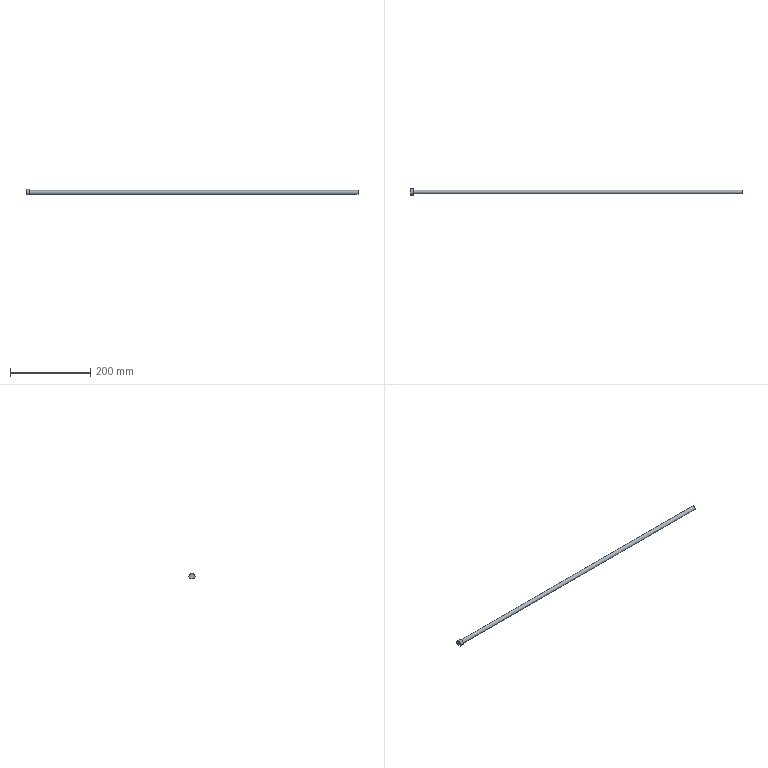Part | STEP file | solid 44 | 1 solid | 6 faces | box 825 x 15 x 13 mm | volume 65469 mm3 | plane 4 | cylinder 2 | commonest cylinder face diameters 10 x1 15 x1